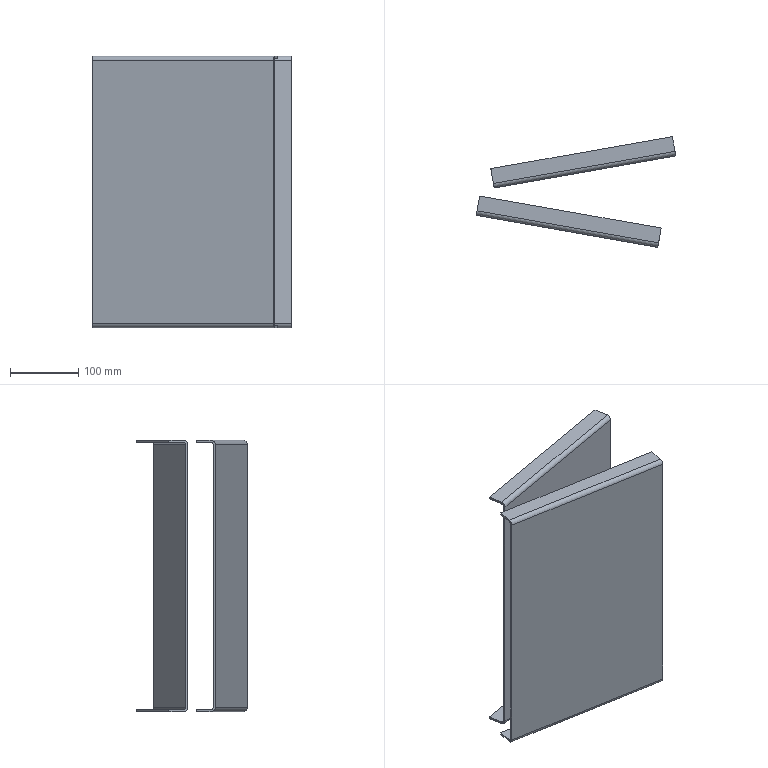Part | NX | features material feeder 3 | 2 solids | 28 faces | box 291.042 x 161.028 x 396 mm | volume 713843 mm3 | plane 20 | cylinder 8 | commonest cylinder face diameters 6 x4 12 x4
STEP:
#1=CARTESIAN_POINT('',(289.479,89.681,-195.));
#2=VERTEX_POINT('',#1);
#3=CARTESIAN_POINT('',(24.479,42.954,-195.));
#4=VERTEX_POINT('',#3);
#5=CARTESIAN_POINT('',(289.479,89.681,-195.));
#6=DIRECTION('',(-0.9848,-0.1736,0.));
#7=VECTOR('',#6,1000.);
#8=LINE('',#5,#7);
#9=EDGE_CURVE('',#2,#4,#8,.T.);
#10=ORIENTED_EDGE('',*,*,#9,.T.);
#11=CARTESIAN_POINT('',(25.,40.,-192.));
#12=VERTEX_POINT('',#11);
#13=CARTESIAN_POINT('',(24.479,42.954,-192.));
#14=DIRECTION('',(0.9848,0.1736,0.));
#15=DIRECTION('',(-0.1736,0.9848,0.));
#16=AXIS2_PLACEMENT_3D('',#13,#14,#15);
#17=CIRCLE('',#16,3.);
#18=EDGE_CURVE('',#12,#4,#17,.T.);
#19=ORIENTED_EDGE('',*,*,#18,.F.);
#20=CARTESIAN_POINT('',(290.,86.727,-192.));
#21=VERTEX_POINT('',#20);
#22=CARTESIAN_POINT('',(25.,40.,-192.));
#23=DIRECTION('',(-0.9848,-0.1736,0.));
#24=VECTOR('',#23,1000.);
#25=LINE('',#22,#24);
#26=EDGE_CURVE('',#21,#12,#25,.T.);
#27=ORIENTED_EDGE('',*,*,#26,.F.);
#28=CARTESIAN_POINT('',(289.479,89.681,-192.));
#29=DIRECTION('',(0.9848,0.1736,0.));
#30=DIRECTION('',(-0.1736,0.9848,0.));
#31=AXIS2_PLACEMENT_3D('',#28,#29,#30);
#32=CIRCLE('',#31,3.);
#33=EDGE_CURVE('',#2,#21,#32,.F.);
#34=ORIENTED_EDGE('',*,*,#33,.F.);
#35=EDGE_LOOP('',(#10,#19,#27,#34));
#36=FACE_BOUND('',#35,.T.);
#37=CARTESIAN_POINT('',(289.479,89.681,-192.));
#38=DIRECTION('',(0.9848,0.1736,0.));
#39=DIRECTION('',(-0.1736,0.9848,0.));
#40=AXIS2_PLACEMENT_3D('',#37,#38,#39);
#41=CYLINDRICAL_SURFACE('',#40,3.);
#42=ADVANCED_FACE('',(#36),#41,.F.);
#43=CARTESIAN_POINT('',(25.,40.,192.));
#44=VERTEX_POINT('',#43);
#45=CARTESIAN_POINT('',(25.,40.,-195.));
#46=DIRECTION('',(0.,0.,1.));
#47=VECTOR('',#46,1000.);
#48=LINE('',#45,#47);
#49=EDGE_CURVE('',#44,#12,#48,.F.);
#50=ORIENTED_EDGE('',*,*,#49,.F.);
#51=CARTESIAN_POINT('',(290.,86.727,192.));
#52=VERTEX_POINT('',#51);
#53=CARTESIAN_POINT('',(25.,40.,192.));
#54=DIRECTION('',(-0.9848,-0.1736,0.));
#55=VECTOR('',#54,1000.);
#56=LINE('',#53,#55);
#57=EDGE_CURVE('',#44,#52,#56,.F.);
#58=ORIENTED_EDGE('',*,*,#57,.T.);
#59=CARTESIAN_POINT('',(290.,86.727,-192.));
#60=DIRECTION('',(0.,0.,1.));
#61=VECTOR('',#60,1000.);
#62=LINE('',#59,#61);
#63=EDGE_CURVE('',#21,#52,#62,.T.);
#64=ORIENTED_EDGE('',*,*,#63,.F.);
#65=ORIENTED_EDGE('',*,*,#26,.T.);
#66=EDGE_LOOP('',(#50,#58,#64,#65));
#67=FACE_BOUND('',#66,.T.);
#68=CARTESIAN_POINT('',(25.,40.,195.));
#69=DIRECTION('',(-0.1736,0.9848,0.));
#70=DIRECTION('',(-0.9848,-0.1736,0.));
#71=AXIS2_PLACEMENT_3D('',#68,#69,#70);
#72=PLANE('',#71);
#73=ADVANCED_FACE('',(#67),#72,.T.);
#74=CARTESIAN_POINT('',(24.479,42.954,195.));
#75=VERTEX_POINT('',#74);
#76=CARTESIAN_POINT('',(289.479,89.681,195.));
#77=VERTEX_POINT('',#76);
#78=CARTESIAN_POINT('',(24.479,42.954,195.));
#79=DIRECTION('',(0.9848,0.1736,0.));
#80=VECTOR('',#79,1000.);
#81=LINE('',#78,#80);
#82=EDGE_CURVE('',#75,#77,#81,.T.);
#83=ORIENTED_EDGE('',*,*,#82,.T.);
#84=CARTESIAN_POINT('',(289.479,89.681,192.));
#85=DIRECTION('',(-0.9848,-0.1736,0.));
#86=DIRECTION('',(0.1736,-0.9848,0.));
#87=AXIS2_PLACEMENT_3D('',#84,#85,#86);
#88=CIRCLE('',#87,3.);
#89=EDGE_CURVE('',#52,#77,#88,.T.);
#90=ORIENTED_EDGE('',*,*,#89,.F.);
#91=ORIENTED_EDGE('',*,*,#57,.F.);
#92=CARTESIAN_POINT('',(24.479,42.954,192.));
#93=DIRECTION('',(-0.9848,-0.1736,0.));
#94=DIRECTION('',(0.1736,-0.9848,0.));
#95=AXIS2_PLACEMENT_3D('',#92,#93,#94);
#96=CIRCLE('',#95,3.);
#97=EDGE_CURVE('',#75,#44,#96,.F.);
#98=ORIENTED_EDGE('',*,*,#97,.F.);
#99=EDGE_LOOP('',(#83,#90,#91,#98));
#100=FACE_BOUND('',#99,.T.);
#101=CARTESIAN_POINT('',(24.479,42.954,192.));
#102=DIRECTION('',(-0.9848,-0.1736,0.));
#103=DIRECTION('',(0.1736,-0.9848,0.));
#104=AXIS2_PLACEMENT_3D('',#101,#102,#103);
#105=CYLINDRICAL_SURFACE('',#104,3.);
#106=ADVANCED_FACE('',(#100),#105,.F.);
#107=CARTESIAN_POINT('',(285.659,111.347,195.));
#108=VERTEX_POINT('',#107);
#109=CARTESIAN_POINT('',(20.659,64.62,195.));
#110=VERTEX_POINT('',#109);
#111=CARTESIAN_POINT('',(153.159,87.984,195.));
#112=DIRECTION('',(-0.9848,-0.1736,0.));
#113=VECTOR('',#112,1000.);
#114=LINE('',#111,#113);
#115=EDGE_CURVE('',#108,#110,#114,.T.);
#116=ORIENTED_EDGE('',*,*,#115,.F.);
#117=CARTESIAN_POINT('',(289.479,89.681,195.));
#118=DIRECTION('',(-0.1736,0.9848,0.));
#119=VECTOR('',#118,1000.);
#120=LINE('',#117,#119);
#121=EDGE_CURVE('',#77,#108,#120,.T.);
#122=ORIENTED_EDGE('',*,*,#121,.F.);
#123=ORIENTED_EDGE('',*,*,#82,.F.);
#124=CARTESIAN_POINT('',(22.829,52.31,195.));
#125=DIRECTION('',(0.1736,-0.9848,0.));
#126=VECTOR('',#125,1000.);
#127=LINE('',#124,#126);
#128=EDGE_CURVE('',#110,#75,#127,.T.);
#129=ORIENTED_EDGE('',*,*,#128,.F.);
#130=EDGE_LOOP('',(#116,#122,#123,#129));
#131=FACE_BOUND('',#130,.T.);
#132=CARTESIAN_POINT('',(25.,40.,195.));
#133=DIRECTION('',(0.,0.,1.));
#134=DIRECTION('',(0.,-1.,0.));
#135=AXIS2_PLACEMENT_3D('',#132,#133,#134);
#136=PLANE('',#135);
#137=ADVANCED_FACE('',(#131),#136,.F.);
#138=CARTESIAN_POINT('',(20.659,64.62,198.));
#139=VERTEX_POINT('',#138);
#140=CARTESIAN_POINT('',(20.659,64.62,-195.));
#141=DIRECTION('',(0.,0.,1.));
#142=VECTOR('',#141,1000.);
#143=LINE('',#140,#142);
#144=EDGE_CURVE('',#139,#110,#143,.F.);
#145=ORIENTED_EDGE('',*,*,#144,.F.);
#146=CARTESIAN_POINT('',(285.659,111.347,198.));
#147=VERTEX_POINT('',#146);
#148=CARTESIAN_POINT('',(285.659,111.347,198.));
#149=DIRECTION('',(-0.9848,-0.1736,0.));
#150=VECTOR('',#149,1000.);
#151=LINE('',#148,#150);
#152=EDGE_CURVE('',#147,#139,#151,.T.);
#153=ORIENTED_EDGE('',*,*,#152,.F.);
#154=CARTESIAN_POINT('',(285.659,111.347,-192.));
#155=DIRECTION('',(0.,0.,1.));
#156=VECTOR('',#155,1000.);
#157=LINE('',#154,#156);
#158=EDGE_CURVE('',#108,#147,#157,.T.);
#159=ORIENTED_EDGE('',*,*,#158,.F.);
#160=ORIENTED_EDGE('',*,*,#115,.T.);
#161=EDGE_LOOP('',(#145,#153,#159,#160));
#162=FACE_BOUND('',#161,.T.);
#163=CARTESIAN_POINT('',(153.159,87.984,195.));
#164=DIRECTION('',(-0.1736,0.9848,0.));
#165=DIRECTION('',(-0.9848,-0.1736,0.));
#166=AXIS2_PLACEMENT_3D('',#163,#164,#165);
#167=PLANE('',#166);
#168=ADVANCED_FACE('',(#162),#167,.T.);
#169=CARTESIAN_POINT('',(289.479,89.681,198.));
#170=VERTEX_POINT('',#169);
#171=CARTESIAN_POINT('',(289.479,89.681,198.));
#172=DIRECTION('',(-0.1736,0.9848,0.));
#173=VECTOR('',#172,1000.);
#174=LINE('',#171,#173);
#175=EDGE_CURVE('',#147,#170,#174,.F.);
#176=ORIENTED_EDGE('',*,*,#175,.F.);
#177=ORIENTED_EDGE('',*,*,#152,.T.);
#178=CARTESIAN_POINT('',(24.479,42.954,198.));
#179=VERTEX_POINT('',#178);
#180=CARTESIAN_POINT('',(22.829,52.31,198.));
#181=DIRECTION('',(0.1736,-0.9848,0.));
#182=VECTOR('',#181,1000.);
#183=LINE('',#180,#182);
#184=EDGE_CURVE('',#179,#139,#183,.F.);
#185=ORIENTED_EDGE('',*,*,#184,.F.);
#186=CARTESIAN_POINT('',(24.479,42.954,198.));
#187=DIRECTION('',(-0.9848,-0.1736,0.));
#188=VECTOR('',#187,1000.);
#189=LINE('',#186,#188);
#190=EDGE_CURVE('',#170,#179,#189,.T.);
#191=ORIENTED_EDGE('',*,*,#190,.F.);
#192=EDGE_LOOP('',(#176,#177,#185,#191));
#193=FACE_BOUND('',#192,.T.);
#194=CARTESIAN_POINT('',(25.,40.,198.));
#195=DIRECTION('',(0.,0.,1.));
#196=DIRECTION('',(0.,-1.,0.));
#197=AXIS2_PLACEMENT_3D('',#194,#195,#196);
#198=PLANE('',#197);
#199=ADVANCED_FACE('',(#193),#198,.T.);
#200=CARTESIAN_POINT('',(20.659,64.62,-198.));
#201=VERTEX_POINT('',#200);
#202=CARTESIAN_POINT('',(24.479,42.954,-198.));
#203=VERTEX_POINT('',#202);
#204=CARTESIAN_POINT('',(22.829,52.31,-198.));
#205=DIRECTION('',(0.1736,-0.9848,0.));
#206=VECTOR('',#205,1000.);
#207=LINE('',#204,#206);
#208=EDGE_CURVE('',#201,#203,#207,.T.);
#209=ORIENTED_EDGE('',*,*,#208,.F.);
#210=CARTESIAN_POINT('',(285.659,111.347,-198.));
#211=VERTEX_POINT('',#210);
#212=CARTESIAN_POINT('',(153.159,87.984,-198.));
#213=DIRECTION('',(-0.9848,-0.1736,0.));
#214=VECTOR('',#213,1000.);
#215=LINE('',#212,#214);
#216=EDGE_CURVE('',#211,#201,#215,.T.);
#217=ORIENTED_EDGE('',*,*,#216,.F.);
#218=CARTESIAN_POINT('',(289.479,89.681,-198.));
#219=VERTEX_POINT('',#218);
#220=CARTESIAN_POINT('',(289.479,89.681,-198.));
#221=DIRECTION('',(-0.1736,0.9848,0.));
#222=VECTOR('',#221,1000.);
#223=LINE('',#220,#222);
#224=EDGE_CURVE('',#219,#211,#223,.T.);
#225=ORIENTED_EDGE('',*,*,#224,.F.);
#226=CARTESIAN_POINT('',(289.479,89.681,-198.));
#227=DIRECTION('',(0.9848,0.1736,0.));
#228=VECTOR('',#227,1000.);
#229=LINE('',#226,#228);
#230=EDGE_CURVE('',#203,#219,#229,.T.);
#231=ORIENTED_EDGE('',*,*,#230,.F.);
#232=EDGE_LOOP('',(#209,#217,#225,#231));
#233=FACE_BOUND('',#232,.T.);
#234=CARTESIAN_POINT('',(290.,86.727,-198.));
#235=DIRECTION('',(0.,0.,-1.));
#236=DIRECTION('',(0.,1.,0.));
#237=AXIS2_PLACEMENT_3D('',#234,#235,#236);
#238=PLANE('',#237);
#239=ADVANCED_FACE('',(#233),#238,.T.);
#240=CARTESIAN_POINT('',(285.659,111.347,-195.));
#241=VERTEX_POINT('',#240);
#242=CARTESIAN_POINT('',(285.659,111.347,-192.));
#243=DIRECTION('',(0.,0.,1.));
#244=VECTOR('',#243,1000.);
#245=LINE('',#242,#244);
#246=EDGE_CURVE('',#211,#241,#245,.T.);
#247=ORIENTED_EDGE('',*,*,#246,.F.);
#248=ORIENTED_EDGE('',*,*,#216,.T.);
#249=CARTESIAN_POINT('',(20.659,64.62,-195.));
#250=VERTEX_POINT('',#249);
#251=CARTESIAN_POINT('',(20.659,64.62,-195.));
#252=DIRECTION('',(0.,0.,1.));
#253=VECTOR('',#252,1000.);
#254=LINE('',#251,#253);
#255=EDGE_CURVE('',#250,#201,#254,.F.);
#256=ORIENTED_EDGE('',*,*,#255,.F.);
#257=CARTESIAN_POINT('',(20.659,64.62,-195.));
#258=DIRECTION('',(0.9848,0.1736,0.));
#259=VECTOR('',#258,1000.);
#260=LINE('',#257,#259);
#261=EDGE_CURVE('',#250,#241,#260,.T.);
#262=ORIENTED_EDGE('',*,*,#261,.T.);
#263=EDGE_LOOP('',(#247,#248,#256,#262));
#264=FACE_BOUND('',#263,.T.);
#265=CARTESIAN_POINT('',(153.159,87.984,-195.));
#266=DIRECTION('',(-0.1736,0.9848,0.));
#267=DIRECTION('',(-0.9848,-0.1736,0.));
#268=AXIS2_PLACEMENT_3D('',#265,#266,#267);
#269=PLANE('',#268);
#270=ADVANCED_FACE('',(#264),#269,.T.);
#271=ORIENTED_EDGE('',*,*,#261,.F.);
#272=CARTESIAN_POINT('',(22.829,52.31,-195.));
#273=DIRECTION('',(0.1736,-0.9848,0.));
#274=VECTOR('',#273,1000.);
#275=LINE('',#272,#274);
#276=EDGE_CURVE('',#4,#250,#275,.F.);
#277=ORIENTED_EDGE('',*,*,#276,.F.);
#278=ORIENTED_EDGE('',*,*,#9,.F.);
#279=CARTESIAN_POINT('',(289.479,89.681,-195.));
#280=DIRECTION('',(-0.1736,0.9848,0.));
#281=VECTOR('',#280,1000.);
#282=LINE('',#279,#281);
#283=EDGE_CURVE('',#241,#2,#282,.F.);
#284=ORIENTED_EDGE('',*,*,#283,.F.);
#285=EDGE_LOOP('',(#271,#277,#278,#284));
#286=FACE_BOUND('',#285,.T.);
#287=CARTESIAN_POINT('',(290.,86.727,-195.));
#288=DIRECTION('',(0.,0.,-1.));
#289=DIRECTION('',(0.,1.,0.));
#290=AXIS2_PLACEMENT_3D('',#287,#288,#289);
#291=PLANE('',#290);
#292=ADVANCED_FACE('',(#286),#291,.F.);
#293=CARTESIAN_POINT('',(25.521,37.046,-192.));
#294=VERTEX_POINT('',#293);
#295=CARTESIAN_POINT('',(24.479,42.954,-192.));
#296=DIRECTION('',(0.9848,0.1736,0.));
#297=DIRECTION('',(-0.1736,0.9848,0.));
#298=AXIS2_PLACEMENT_3D('',#295,#296,#297);
#299=CIRCLE('',#298,6.);
#300=EDGE_CURVE('',#203,#294,#299,.F.);
#301=ORIENTED_EDGE('',*,*,#300,.F.);
#302=ORIENTED_EDGE('',*,*,#230,.T.);
#303=CARTESIAN_POINT('',(290.521,83.772,-192.));
#304=VERTEX_POINT('',#303);
#305=CARTESIAN_POINT('',(289.479,89.681,-192.));
#306=DIRECTION('',(0.9848,0.1736,0.));
#307=DIRECTION('',(-0.1736,0.9848,0.));
#308=AXIS2_PLACEMENT_3D('',#305,#306,#307);
#309=CIRCLE('',#308,6.);
#310=EDGE_CURVE('',#304,#219,#309,.T.);
#311=ORIENTED_EDGE('',*,*,#310,.F.);
#312=CARTESIAN_POINT('',(25.521,37.046,-192.));
#313=DIRECTION('',(-0.9848,-0.1736,0.));
#314=VECTOR('',#313,1000.);
#315=LINE('',#312,#314);
#316=EDGE_CURVE('',#304,#294,#315,.T.);
#317=ORIENTED_EDGE('',*,*,#316,.T.);
#318=EDGE_LOOP('',(#301,#302,#311,#317));
#319=FACE_BOUND('',#318,.T.);
#320=CARTESIAN_POINT('',(289.479,89.681,-192.));
#321=DIRECTION('',(0.9848,0.1736,0.));
#322=DIRECTION('',(-0.1736,0.9848,0.));
#323=AXIS2_PLACEMENT_3D('',#320,#321,#322);
#324=CYLINDRICAL_SURFACE('',#323,6.);
#325=ADVANCED_FACE('',(#319),#324,.T.);
#326=ORIENTED_EDGE('',*,*,#276,.T.);
#327=ORIENTED_EDGE('',*,*,#255,.T.);
#328=ORIENTED_EDGE('',*,*,#208,.T.);
#329=ORIENTED_EDGE('',*,*,#300,.T.);
#330=CARTESIAN_POINT('',(25.521,37.046,192.));
#331=VERTEX_POINT('',#330);
#332=CARTESIAN_POINT('',(25.521,37.046,195.));
#333=DIRECTION('',(0.,0.,1.));
#334=VECTOR('',#333,1000.);
#335=LINE('',#332,#334);
#336=EDGE_CURVE('',#294,#331,#335,.T.);
#337=ORIENTED_EDGE('',*,*,#336,.T.);
#338=CARTESIAN_POINT('',(24.479,42.954,192.));
#339=DIRECTION('',(-0.9848,-0.1736,0.));
#340=DIRECTION('',(0.1736,-0.9848,0.));
#341=AXIS2_PLACEMENT_3D('',#338,#339,#340);
#342=CIRCLE('',#341,6.);
#343=EDGE_CURVE('',#179,#331,#342,.F.);
#344=ORIENTED_EDGE('',*,*,#343,.F.);
#345=ORIENTED_EDGE('',*,*,#184,.T.);
#346=ORIENTED_EDGE('',*,*,#144,.T.);
#347=ORIENTED_EDGE('',*,*,#128,.T.);
#348=ORIENTED_EDGE('',*,*,#97,.T.);
#349=ORIENTED_EDGE('',*,*,#49,.T.);
#350=ORIENTED_EDGE('',*,*,#18,.T.);
#351=EDGE_LOOP('',(#326,#327,#328,#329,#337,#344,#345,#346,#347,#348,#349,#350));
#352=FACE_BOUND('',#351,.T.);
#353=CARTESIAN_POINT('',(22.829,52.31,-195.));
#354=DIRECTION('',(-0.9848,-0.1736,0.));
#355=DIRECTION('',(0.1736,-0.9848,0.));
#356=AXIS2_PLACEMENT_3D('',#353,#354,#355);
#357=PLANE('',#356);
#358=ADVANCED_FACE('',(#352),#357,.T.);
#359=CARTESIAN_POINT('',(290.521,83.772,192.));
#360=VERTEX_POINT('',#359);
#361=CARTESIAN_POINT('',(289.479,89.681,192.));
#362=DIRECTION('',(-0.9848,-0.1736,0.));
#363=DIRECTION('',(0.1736,-0.9848,0.));
#364=AXIS2_PLACEMENT_3D('',#361,#362,#363);
#365=CIRCLE('',#364,6.);
#366=EDGE_CURVE('',#170,#360,#365,.F.);
#367=ORIENTED_EDGE('',*,*,#366,.F.);
#368=ORIENTED_EDGE('',*,*,#190,.T.);
#369=ORIENTED_EDGE('',*,*,#343,.T.);
#370=CARTESIAN_POINT('',(25.521,37.046,192.));
#371=DIRECTION('',(-0.9848,-0.1736,0.));
#372=VECTOR('',#371,1000.);
#373=LINE('',#370,#372);
#374=EDGE_CURVE('',#331,#360,#373,.F.);
#375=ORIENTED_EDGE('',*,*,#374,.T.);
#376=EDGE_LOOP('',(#367,#368,#369,#375));
#377=FACE_BOUND('',#376,.T.);
#378=CARTESIAN_POINT('',(24.479,42.954,192.));
#379=DIRECTION('',(-0.9848,-0.1736,0.));
#380=DIRECTION('',(0.1736,-0.9848,0.));
#381=AXIS2_PLACEMENT_3D('',#378,#379,#380);
#382=CYLINDRICAL_SURFACE('',#381,6.);
#383=ADVANCED_FACE('',(#377),#382,.T.);
#384=ORIENTED_EDGE('',*,*,#246,.T.);
#385=ORIENTED_EDGE('',*,*,#283,.T.);
#386=ORIENTED_EDGE('',*,*,#33,.T.);
#387=ORIENTED_EDGE('',*,*,#63,.T.);
#388=ORIENTED_EDGE('',*,*,#89,.T.);
#389=ORIENTED_EDGE('',*,*,#121,.T.);
#390=ORIENTED_EDGE('',*,*,#158,.T.);
#391=ORIENTED_EDGE('',*,*,#175,.T.);
#392=ORIENTED_EDGE('',*,*,#366,.T.);
#393=CARTESIAN_POINT('',(290.521,83.772,195.));
#394=DIRECTION('',(0.,0.,1.));
#395=VECTOR('',#394,1000.);
#396=LINE('',#393,#395);
#397=EDGE_CURVE('',#360,#304,#396,.F.);
#398=ORIENTED_EDGE('',*,*,#397,.T.);
#399=ORIENTED_EDGE('',*,*,#310,.T.);
#400=ORIENTED_EDGE('',*,*,#224,.T.);
#401=EDGE_LOOP('',(#384,#385,#386,#387,#388,#389,#390,#391,#392,#398,#399,#400));
#402=FACE_BOUND('',#401,.T.);
#403=CARTESIAN_POINT('',(289.479,89.681,-192.));
#404=DIRECTION('',(0.9848,0.1736,0.));
#405=DIRECTION('',(-0.1736,0.9848,0.));
#406=AXIS2_PLACEMENT_3D('',#403,#404,#405);
#407=PLANE('',#406);
#408=ADVANCED_FACE('',(#402),#407,.T.);
#409=ORIENTED_EDGE('',*,*,#374,.F.);
#410=ORIENTED_EDGE('',*,*,#336,.F.);
#411=ORIENTED_EDGE('',*,*,#316,.F.);
#412=ORIENTED_EDGE('',*,*,#397,.F.);
#413=EDGE_LOOP('',(#409,#410,#411,#412));
#414=FACE_BOUND('',#413,.T.);
#415=CARTESIAN_POINT('',(25.521,37.046,195.));
#416=DIRECTION('',(-0.1736,0.9848,0.));
#417=DIRECTION('',(-0.9848,-0.1736,0.));
#418=AXIS2_PLACEMENT_3D('',#415,#416,#417);
#419=PLANE('',#418);
#420=ADVANCED_FACE('',(#414),#419,.F.);
#421=CLOSED_SHELL('',(#42,#73,#106,#137,#168,#199,#239,#270,#292,#325,#358,#383,#408,#420));
#422=MANIFOLD_SOLID_BREP('',#421);
#423=CARTESIAN_POINT('',(269.341,-22.106,-198.));
#424=VERTEX_POINT('',#423);
#425=CARTESIAN_POINT('',(4.341,24.62,-198.));
#426=VERTEX_POINT('',#425);
#427=CARTESIAN_POINT('',(136.841,1.257,-198.));
#428=DIRECTION('',(-0.9848,0.1736,0.));
#429=VECTOR('',#428,1000.);
#430=LINE('',#427,#429);
#431=EDGE_CURVE('',#424,#426,#430,.T.);
#432=ORIENTED_EDGE('',*,*,#431,.F.);
#433=CARTESIAN_POINT('',(265.521,-43.772,-198.));
#434=VERTEX_POINT('',#433);
#435=CARTESIAN_POINT('',(267.171,-34.417,-198.));
#436=DIRECTION('',(0.1736,0.9848,0.));
#437=VECTOR('',#436,1000.);
#438=LINE('',#435,#437);
#439=EDGE_CURVE('',#434,#424,#438,.T.);
#440=ORIENTED_EDGE('',*,*,#439,.F.);
#441=CARTESIAN_POINT('',(0.5209,2.954,-198.));
#442=VERTEX_POINT('',#441);
#443=CARTESIAN_POINT('',(0.5209,2.954,-198.));
#444=DIRECTION('',(0.9848,-0.1736,0.));
#445=VECTOR('',#444,1000.);
#446=LINE('',#443,#445);
#447=EDGE_CURVE('',#442,#434,#446,.T.);
#448=ORIENTED_EDGE('',*,*,#447,.F.);
#449=CARTESIAN_POINT('',(0.5209,2.954,-198.));
#450=DIRECTION('',(0.1736,0.9848,0.));
#451=VECTOR('',#450,1000.);
#452=LINE('',#449,#451);
#453=EDGE_CURVE('',#442,#426,#452,.T.);
#454=ORIENTED_EDGE('',*,*,#453,.T.);
#455=EDGE_LOOP('',(#432,#440,#448,#454));
#456=FACE_BOUND('',#455,.T.);
#457=CARTESIAN_POINT('',(0.,0.,-198.));
#458=DIRECTION('',(0.,0.,1.));
#459=DIRECTION('',(0.,-1.,0.));
#460=AXIS2_PLACEMENT_3D('',#457,#458,#459);
#461=PLANE('',#460);
#462=ADVANCED_FACE('',(#456),#461,.F.);
#463=CARTESIAN_POINT('',(4.341,24.62,-195.));
#464=VERTEX_POINT('',#463);
#465=CARTESIAN_POINT('',(4.341,24.62,-192.));
#466=DIRECTION('',(0.,0.,1.));
#467=VECTOR('',#466,1000.);
#468=LINE('',#465,#467);
#469=EDGE_CURVE('',#426,#464,#468,.T.);
#470=ORIENTED_EDGE('',*,*,#469,.T.);
#471=CARTESIAN_POINT('',(269.341,-22.106,-195.));
#472=VERTEX_POINT('',#471);
#473=CARTESIAN_POINT('',(269.341,-22.106,-195.));
#474=DIRECTION('',(-0.9848,0.1736,0.));
#475=VECTOR('',#474,1000.);
#476=LINE('',#473,#475);
#477=EDGE_CURVE('',#472,#464,#476,.T.);
#478=ORIENTED_EDGE('',*,*,#477,.F.);
#479=CARTESIAN_POINT('',(269.341,-22.106,-195.));
#480=DIRECTION('',(0.,0.,1.));
#481=VECTOR('',#480,1000.);
#482=LINE('',#479,#481);
#483=EDGE_CURVE('',#424,#472,#482,.T.);
#484=ORIENTED_EDGE('',*,*,#483,.F.);
#485=ORIENTED_EDGE('',*,*,#431,.T.);
#486=EDGE_LOOP('',(#470,#478,#484,#485));
#487=FACE_BOUND('',#486,.T.);
#488=CARTESIAN_POINT('',(136.841,1.257,-195.));
#489=DIRECTION('',(0.1736,0.9848,0.));
#490=DIRECTION('',(-0.9848,0.1736,0.));
#491=AXIS2_PLACEMENT_3D('',#488,#489,#490);
#492=PLANE('',#491);
#493=ADVANCED_FACE('',(#487),#492,.T.);
#494=CARTESIAN_POINT('',(265.521,-43.772,-195.));
#495=VERTEX_POINT('',#494);
#496=CARTESIAN_POINT('',(267.171,-34.417,-195.));
#497=DIRECTION('',(0.1736,0.9848,0.));
#498=VECTOR('',#497,1000.);
#499=LINE('',#496,#498);
#500=EDGE_CURVE('',#472,#495,#499,.F.);
#501=ORIENTED_EDGE('',*,*,#500,.F.);
#502=ORIENTED_EDGE('',*,*,#477,.T.);
#503=CARTESIAN_POINT('',(0.5209,2.954,-195.));
#504=VERTEX_POINT('',#503);
#505=CARTESIAN_POINT('',(0.5209,2.954,-195.));
#506=DIRECTION('',(0.1736,0.9848,0.));
#507=VECTOR('',#506,1000.);
#508=LINE('',#505,#507);
#509=EDGE_CURVE('',#464,#504,#508,.F.);
#510=ORIENTED_EDGE('',*,*,#509,.T.);
#511=CARTESIAN_POINT('',(0.5209,2.954,-195.));
#512=DIRECTION('',(0.9848,-0.1736,0.));
#513=VECTOR('',#512,1000.);
#514=LINE('',#511,#513);
#515=EDGE_CURVE('',#504,#495,#514,.T.);
#516=ORIENTED_EDGE('',*,*,#515,.T.);
#517=EDGE_LOOP('',(#501,#502,#510,#516));
#518=FACE_BOUND('',#517,.T.);
#519=CARTESIAN_POINT('',(0.,0.,-195.));
#520=DIRECTION('',(0.,0.,1.));
#521=DIRECTION('',(0.,-1.,0.));
#522=AXIS2_PLACEMENT_3D('',#519,#520,#521);
#523=PLANE('',#522);
#524=ADVANCED_FACE('',(#518),#523,.T.);
#525=CARTESIAN_POINT('',(0.5209,2.954,195.));
#526=VERTEX_POINT('',#525);
#527=CARTESIAN_POINT('',(4.341,24.62,195.));
#528=VERTEX_POINT('',#527);
#529=CARTESIAN_POINT('',(0.5209,2.954,195.));
#530=DIRECTION('',(0.1736,0.9848,0.));
#531=VECTOR('',#530,1000.);
#532=LINE('',#529,#531);
#533=EDGE_CURVE('',#526,#528,#532,.T.);
#534=ORIENTED_EDGE('',*,*,#533,.T.);
#535=CARTESIAN_POINT('',(269.341,-22.106,195.));
#536=VERTEX_POINT('',#535);
#537=CARTESIAN_POINT('',(136.841,1.257,195.));
#538=DIRECTION('',(-0.9848,0.1736,0.));
#539=VECTOR('',#538,1000.);
#540=LINE('',#537,#539);
#541=EDGE_CURVE('',#536,#528,#540,.T.);
#542=ORIENTED_EDGE('',*,*,#541,.F.);
#543=CARTESIAN_POINT('',(265.521,-43.772,195.));
#544=VERTEX_POINT('',#543);
#545=CARTESIAN_POINT('',(267.171,-34.417,195.));
#546=DIRECTION('',(0.1736,0.9848,0.));
#547=VECTOR('',#546,1000.);
#548=LINE('',#545,#547);
#549=EDGE_CURVE('',#544,#536,#548,.T.);
#550=ORIENTED_EDGE('',*,*,#549,.F.);
#551=CARTESIAN_POINT('',(265.521,-43.772,195.));
#552=DIRECTION('',(-0.9848,0.1736,0.));
#553=VECTOR('',#552,1000.);
#554=LINE('',#551,#553);
#555=EDGE_CURVE('',#544,#526,#554,.T.);
#556=ORIENTED_EDGE('',*,*,#555,.T.);
#557=EDGE_LOOP('',(#534,#542,#550,#556));
#558=FACE_BOUND('',#557,.T.);
#559=CARTESIAN_POINT('',(265.,-46.727,195.));
#560=DIRECTION('',(0.,0.,-1.));
#561=DIRECTION('',(0.,1.,0.));
#562=AXIS2_PLACEMENT_3D('',#559,#560,#561);
#563=PLANE('',#562);
#564=ADVANCED_FACE('',(#558),#563,.T.);
#565=CARTESIAN_POINT('',(269.341,-22.106,198.));
#566=VERTEX_POINT('',#565);
#567=CARTESIAN_POINT('',(269.341,-22.106,-195.));
#568=DIRECTION('',(0.,0.,1.));
#569=VECTOR('',#568,1000.);
#570=LINE('',#567,#569);
#571=EDGE_CURVE('',#536,#566,#570,.T.);
#572=ORIENTED_EDGE('',*,*,#571,.F.);
#573=ORIENTED_EDGE('',*,*,#541,.T.);
#574=CARTESIAN_POINT('',(4.341,24.62,198.));
#575=VERTEX_POINT('',#574);
#576=CARTESIAN_POINT('',(4.341,24.62,-192.));
#577=DIRECTION('',(0.,0.,1.));
#578=VECTOR('',#577,1000.);
#579=LINE('',#576,#578);
#580=EDGE_CURVE('',#528,#575,#579,.T.);
#581=ORIENTED_EDGE('',*,*,#580,.T.);
#582=CARTESIAN_POINT('',(4.341,24.62,198.));
#583=DIRECTION('',(0.9848,-0.1736,0.));
#584=VECTOR('',#583,1000.);
#585=LINE('',#582,#584);
#586=EDGE_CURVE('',#575,#566,#585,.T.);
#587=ORIENTED_EDGE('',*,*,#586,.T.);
#588=EDGE_LOOP('',(#572,#573,#581,#587));
#589=FACE_BOUND('',#588,.T.);
#590=CARTESIAN_POINT('',(136.841,1.257,195.));
#591=DIRECTION('',(0.1736,0.9848,0.));
#592=DIRECTION('',(-0.9848,0.1736,0.));
#593=AXIS2_PLACEMENT_3D('',#590,#591,#592);
#594=PLANE('',#593);
#595=ADVANCED_FACE('',(#589),#594,.T.);
#596=ORIENTED_EDGE('',*,*,#586,.F.);
#597=CARTESIAN_POINT('',(0.5209,2.954,198.));
#598=VERTEX_POINT('',#597);
#599=CARTESIAN_POINT('',(0.5209,2.954,198.));
#600=DIRECTION('',(0.1736,0.9848,0.));
#601=VECTOR('',#600,1000.);
#602=LINE('',#599,#601);
#603=EDGE_CURVE('',#575,#598,#602,.F.);
#604=ORIENTED_EDGE('',*,*,#603,.T.);
#605=CARTESIAN_POINT('',(265.521,-43.772,198.));
#606=VERTEX_POINT('',#605);
#607=CARTESIAN_POINT('',(265.521,-43.772,198.));
#608=DIRECTION('',(-0.9848,0.1736,0.));
#609=VECTOR('',#608,1000.);
#610=LINE('',#607,#609);
#611=EDGE_CURVE('',#606,#598,#610,.T.);
#612=ORIENTED_EDGE('',*,*,#611,.F.);
#613=CARTESIAN_POINT('',(267.171,-34.417,198.));
#614=DIRECTION('',(0.1736,0.9848,0.));
#615=VECTOR('',#614,1000.);
#616=LINE('',#613,#615);
#617=EDGE_CURVE('',#566,#606,#616,.F.);
#618=ORIENTED_EDGE('',*,*,#617,.F.);
#619=EDGE_LOOP('',(#596,#604,#612,#618));
#620=FACE_BOUND('',#619,.T.);
#621=CARTESIAN_POINT('',(265.,-46.727,198.));
#622=DIRECTION('',(0.,0.,-1.));
#623=DIRECTION('',(0.,1.,0.));
#624=AXIS2_PLACEMENT_3D('',#621,#622,#623);
#625=PLANE('',#624);
#626=ADVANCED_FACE('',(#620),#625,.F.);
#627=CARTESIAN_POINT('',(-0.5209,-2.954,192.));
#628=VERTEX_POINT('',#627);
#629=CARTESIAN_POINT('',(0.5209,2.954,192.));
#630=DIRECTION('',(-0.9848,0.1736,0.));
#631=DIRECTION('',(-0.1736,-0.9848,0.));
#632=AXIS2_PLACEMENT_3D('',#629,#630,#631);
#633=CIRCLE('',#632,6.);
#634=EDGE_CURVE('',#598,#628,#633,.F.);
#635=ORIENTED_EDGE('',*,*,#634,.T.);
#636=CARTESIAN_POINT('',(264.479,-49.681,192.));
#637=VERTEX_POINT('',#636);
#638=CARTESIAN_POINT('',(264.479,-49.681,192.));
#639=DIRECTION('',(0.9848,-0.1736,0.));
#640=VECTOR('',#639,1000.);
#641=LINE('',#638,#640);
#642=EDGE_CURVE('',#637,#628,#641,.F.);
#643=ORIENTED_EDGE('',*,*,#642,.F.);
#644=CARTESIAN_POINT('',(265.521,-43.772,192.));
#645=DIRECTION('',(-0.9848,0.1736,0.));
#646=DIRECTION('',(-0.1736,-0.9848,0.));
#647=AXIS2_PLACEMENT_3D('',#644,#645,#646);
#648=CIRCLE('',#647,6.);
#649=EDGE_CURVE('',#606,#637,#648,.F.);
#650=ORIENTED_EDGE('',*,*,#649,.F.);
#651=ORIENTED_EDGE('',*,*,#611,.T.);
#652=EDGE_LOOP('',(#635,#643,#650,#651));
#653=FACE_BOUND('',#652,.T.);
#654=CARTESIAN_POINT('',(265.521,-43.772,192.));
#655=DIRECTION('',(-0.9848,0.1736,0.));
#656=DIRECTION('',(-0.1736,-0.9848,0.));
#657=AXIS2_PLACEMENT_3D('',#654,#655,#656);
#658=CYLINDRICAL_SURFACE('',#657,6.);
#659=ADVANCED_FACE('',(#653),#658,.T.);
#660=CARTESIAN_POINT('',(264.479,-49.681,-192.));
#661=VERTEX_POINT('',#660);
#662=CARTESIAN_POINT('',(264.479,-49.681,-195.));
#663=DIRECTION('',(0.,0.,1.));
#664=VECTOR('',#663,1000.);
#665=LINE('',#662,#664);
#666=EDGE_CURVE('',#637,#661,#665,.F.);
#667=ORIENTED_EDGE('',*,*,#666,.F.);
#668=ORIENTED_EDGE('',*,*,#642,.T.);
#669=CARTESIAN_POINT('',(-0.5209,-2.954,-192.));
#670=VERTEX_POINT('',#669);
#671=CARTESIAN_POINT('',(-0.5209,-2.954,-192.));
#672=DIRECTION('',(0.,0.,1.));
#673=VECTOR('',#672,1000.);
#674=LINE('',#671,#673);
#675=EDGE_CURVE('',#628,#670,#674,.F.);
#676=ORIENTED_EDGE('',*,*,#675,.T.);
#677=CARTESIAN_POINT('',(-0.5209,-2.954,-192.));
#678=DIRECTION('',(0.9848,-0.1736,0.));
#679=VECTOR('',#678,1000.);
#680=LINE('',#677,#679);
#681=EDGE_CURVE('',#661,#670,#680,.F.);
#682=ORIENTED_EDGE('',*,*,#681,.F.);
#683=EDGE_LOOP('',(#667,#668,#676,#682));
#684=FACE_BOUND('',#683,.T.);
#685=CARTESIAN_POINT('',(264.479,-49.681,195.));
#686=DIRECTION('',(-0.1736,-0.9848,0.));
#687=DIRECTION('',(0.9848,-0.1736,0.));
#688=AXIS2_PLACEMENT_3D('',#685,#686,#687);
#689=PLANE('',#688);
#690=ADVANCED_FACE('',(#684),#689,.T.);
#691=CARTESIAN_POINT('',(265.521,-43.772,-192.));
#692=DIRECTION('',(0.9848,-0.1736,0.));
#693=DIRECTION('',(0.1736,0.9848,0.));
#694=AXIS2_PLACEMENT_3D('',#691,#692,#693);
#695=CIRCLE('',#694,6.);
#696=EDGE_CURVE('',#661,#434,#695,.T.);
#697=ORIENTED_EDGE('',*,*,#696,.F.);
#698=ORIENTED_EDGE('',*,*,#681,.T.);
#699=CARTESIAN_POINT('',(0.5209,2.954,-192.));
#700=DIRECTION('',(0.9848,-0.1736,0.));
#701=DIRECTION('',(0.1736,0.9848,0.));
#702=AXIS2_PLACEMENT_3D('',#699,#700,#701);
#703=CIRCLE('',#702,6.);
#704=EDGE_CURVE('',#670,#442,#703,.T.);
#705=ORIENTED_EDGE('',*,*,#704,.T.);
#706=ORIENTED_EDGE('',*,*,#447,.T.);
#707=EDGE_LOOP('',(#697,#698,#705,#706));
#708=FACE_BOUND('',#707,.T.);
#709=CARTESIAN_POINT('',(0.5209,2.954,-192.));
#710=DIRECTION('',(0.9848,-0.1736,0.));
#711=DIRECTION('',(0.1736,0.9848,0.));
#712=AXIS2_PLACEMENT_3D('',#709,#710,#711);
#713=CYLINDRICAL_SURFACE('',#712,6.);
#714=ADVANCED_FACE('',(#708),#713,.T.);
#715=CARTESIAN_POINT('',(0.,0.,-192.));
#716=VERTEX_POINT('',#715);
#717=CARTESIAN_POINT('',(265.,-46.727,-192.));
#718=VERTEX_POINT('',#717);
#719=CARTESIAN_POINT('',(265.,-46.727,-192.));
#720=DIRECTION('',(0.9848,-0.1736,0.));
#721=VECTOR('',#720,1000.);
#722=LINE('',#719,#721);
#723=EDGE_CURVE('',#716,#718,#722,.T.);
#724=ORIENTED_EDGE('',*,*,#723,.T.);
#725=CARTESIAN_POINT('',(265.521,-43.772,-192.));
#726=DIRECTION('',(0.9848,-0.1736,0.));
#727=DIRECTION('',(0.1736,0.9848,0.));
#728=AXIS2_PLACEMENT_3D('',#725,#726,#727);
#729=CIRCLE('',#728,3.);
#730=EDGE_CURVE('',#495,#718,#729,.F.);
#731=ORIENTED_EDGE('',*,*,#730,.F.);
#732=ORIENTED_EDGE('',*,*,#515,.F.);
#733=CARTESIAN_POINT('',(0.5209,2.954,-192.));
#734=DIRECTION('',(0.9848,-0.1736,0.));
#735=DIRECTION('',(0.1736,0.9848,0.));
#736=AXIS2_PLACEMENT_3D('',#733,#734,#735);
#737=CIRCLE('',#736,3.);
#738=EDGE_CURVE('',#504,#716,#737,.F.);
#739=ORIENTED_EDGE('',*,*,#738,.T.);
#740=EDGE_LOOP('',(#724,#731,#732,#739));
#741=FACE_BOUND('',#740,.T.);
#742=CARTESIAN_POINT('',(0.5209,2.954,-192.));
#743=DIRECTION('',(0.9848,-0.1736,0.));
#744=DIRECTION('',(0.1736,0.9848,0.));
#745=AXIS2_PLACEMENT_3D('',#742,#743,#744);
#746=CYLINDRICAL_SURFACE('',#745,3.);
#747=ADVANCED_FACE('',(#741),#746,.F.);
#748=ORIENTED_EDGE('',*,*,#439,.T.);
#749=ORIENTED_EDGE('',*,*,#483,.T.);
#750=ORIENTED_EDGE('',*,*,#500,.T.);
#751=ORIENTED_EDGE('',*,*,#730,.T.);
#752=CARTESIAN_POINT('',(265.,-46.727,192.));
#753=VERTEX_POINT('',#752);
#754=CARTESIAN_POINT('',(265.,-46.727,195.));
#755=DIRECTION('',(0.,0.,1.));
#756=VECTOR('',#755,1000.);
#757=LINE('',#754,#756);
#758=EDGE_CURVE('',#718,#753,#757,.T.);
#759=ORIENTED_EDGE('',*,*,#758,.T.);
#760=CARTESIAN_POINT('',(265.521,-43.772,192.));
#761=DIRECTION('',(-0.9848,0.1736,0.));
#762=DIRECTION('',(-0.1736,-0.9848,0.));
#763=AXIS2_PLACEMENT_3D('',#760,#761,#762);
#764=CIRCLE('',#763,3.);
#765=EDGE_CURVE('',#753,#544,#764,.T.);
#766=ORIENTED_EDGE('',*,*,#765,.T.);
#767=ORIENTED_EDGE('',*,*,#549,.T.);
#768=ORIENTED_EDGE('',*,*,#571,.T.);
#769=ORIENTED_EDGE('',*,*,#617,.T.);
#770=ORIENTED_EDGE('',*,*,#649,.T.);
#771=ORIENTED_EDGE('',*,*,#666,.T.);
#772=ORIENTED_EDGE('',*,*,#696,.T.);
#773=EDGE_LOOP('',(#748,#749,#750,#751,#759,#766,#767,#768,#769,#770,#771,#772));
#774=FACE_BOUND('',#773,.T.);
#775=CARTESIAN_POINT('',(267.171,-34.417,-195.));
#776=DIRECTION('',(0.9848,-0.1736,0.));
#777=DIRECTION('',(0.1736,0.9848,0.));
#778=AXIS2_PLACEMENT_3D('',#775,#776,#777);
#779=PLANE('',#778);
#780=ADVANCED_FACE('',(#774),#779,.T.);
#781=CARTESIAN_POINT('',(0.,0.,192.));
#782=VERTEX_POINT('',#781);
#783=CARTESIAN_POINT('',(265.,-46.727,192.));
#784=DIRECTION('',(0.9848,-0.1736,0.));
#785=VECTOR('',#784,1000.);
#786=LINE('',#783,#785);
#787=EDGE_CURVE('',#753,#782,#786,.F.);
#788=ORIENTED_EDGE('',*,*,#787,.T.);
#789=CARTESIAN_POINT('',(0.5209,2.954,192.));
#790=DIRECTION('',(-0.9848,0.1736,0.));
#791=DIRECTION('',(-0.1736,-0.9848,0.));
#792=AXIS2_PLACEMENT_3D('',#789,#790,#791);
#793=CIRCLE('',#792,3.);
#794=EDGE_CURVE('',#782,#526,#793,.T.);
#795=ORIENTED_EDGE('',*,*,#794,.T.);
#796=ORIENTED_EDGE('',*,*,#555,.F.);
#797=ORIENTED_EDGE('',*,*,#765,.F.);
#798=EDGE_LOOP('',(#788,#795,#796,#797));
#799=FACE_BOUND('',#798,.T.);
#800=CARTESIAN_POINT('',(265.521,-43.772,192.));
#801=DIRECTION('',(-0.9848,0.1736,0.));
#802=DIRECTION('',(-0.1736,-0.9848,0.));
#803=AXIS2_PLACEMENT_3D('',#800,#801,#802);
#804=CYLINDRICAL_SURFACE('',#803,3.);
#805=ADVANCED_FACE('',(#799),#804,.F.);
#806=ORIENTED_EDGE('',*,*,#675,.F.);
#807=ORIENTED_EDGE('',*,*,#634,.F.);
#808=ORIENTED_EDGE('',*,*,#603,.F.);
#809=ORIENTED_EDGE('',*,*,#580,.F.);
#810=ORIENTED_EDGE('',*,*,#533,.F.);
#811=ORIENTED_EDGE('',*,*,#794,.F.);
#812=CARTESIAN_POINT('',(0.,0.,195.));
#813=DIRECTION('',(0.,0.,1.));
#814=VECTOR('',#813,1000.);
#815=LINE('',#812,#814);
#816=EDGE_CURVE('',#782,#716,#815,.F.);
#817=ORIENTED_EDGE('',*,*,#816,.T.);
#818=ORIENTED_EDGE('',*,*,#738,.F.);
#819=ORIENTED_EDGE('',*,*,#509,.F.);
#820=ORIENTED_EDGE('',*,*,#469,.F.);
#821=ORIENTED_EDGE('',*,*,#453,.F.);
#822=ORIENTED_EDGE('',*,*,#704,.F.);
#823=EDGE_LOOP('',(#806,#807,#808,#809,#810,#811,#817,#818,#819,#820,#821,#822));
#824=FACE_BOUND('',#823,.T.);
#825=CARTESIAN_POINT('',(0.5209,2.954,-192.));
#826=DIRECTION('',(0.9848,-0.1736,0.));
#827=DIRECTION('',(0.1736,0.9848,0.));
#828=AXIS2_PLACEMENT_3D('',#825,#826,#827);
#829=PLANE('',#828);
#830=ADVANCED_FACE('',(#824),#829,.F.);
#831=ORIENTED_EDGE('',*,*,#787,.F.);
#832=ORIENTED_EDGE('',*,*,#758,.F.);
#833=ORIENTED_EDGE('',*,*,#723,.F.);
#834=ORIENTED_EDGE('',*,*,#816,.F.);
#835=EDGE_LOOP('',(#831,#832,#833,#834));
#836=FACE_BOUND('',#835,.T.);
#837=CARTESIAN_POINT('',(265.,-46.727,195.));
#838=DIRECTION('',(-0.1736,-0.9848,0.));
#839=DIRECTION('',(0.9848,-0.1736,0.));
#840=AXIS2_PLACEMENT_3D('',#837,#838,#839);
#841=PLANE('',#840);
#842=ADVANCED_FACE('',(#836),#841,.F.);
#843=CLOSED_SHELL('',(#462,#493,#524,#564,#595,#626,#659,#690,#714,#747,#780,#805,#830,#842));
#844=MANIFOLD_SOLID_BREP('',#843);
#845=(LENGTH_UNIT()NAMED_UNIT(*)SI_UNIT(.MILLI.,.METRE.));
#846=UNCERTAINTY_MEASURE_WITH_UNIT(LENGTH_MEASURE(0.00001),#845,'','');
#847=(NAMED_UNIT(*)PLANE_ANGLE_UNIT()SI_UNIT($,.RADIAN.));
#848=(NAMED_UNIT(*)SI_UNIT($,.STERADIAN.)SOLID_ANGLE_UNIT());
#849=(GEOMETRIC_REPRESENTATION_CONTEXT(3)GLOBAL_UNCERTAINTY_ASSIGNED_CONTEXT((#846))GLOBAL_UNIT_ASSIGNED_CONTEXT((#845,#847,#848))REPRESENTATION_CONTEXT('',''));
#850=ADVANCED_BREP_SHAPE_REPRESENTATION('',(#422,#844),#849);